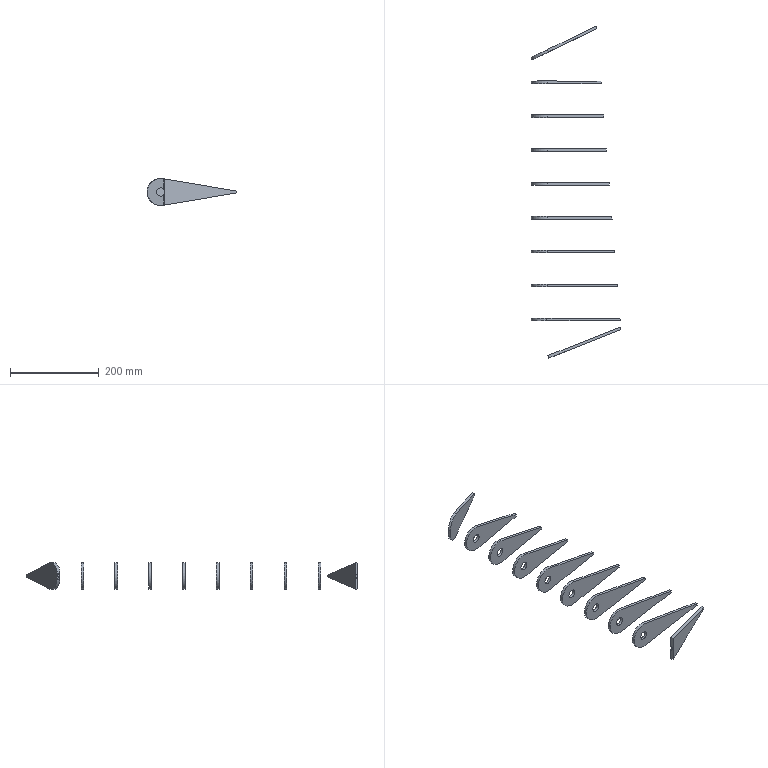Part | SolidWorks | features BaseBody 10 | 10 solids | 69 faces | box 202.602 x 749.483 x 60.961 mm | volume 360036 mm3 | plane 32 | spline 20 | cylinder 17 | commonest cylinder face diameters 19 x17